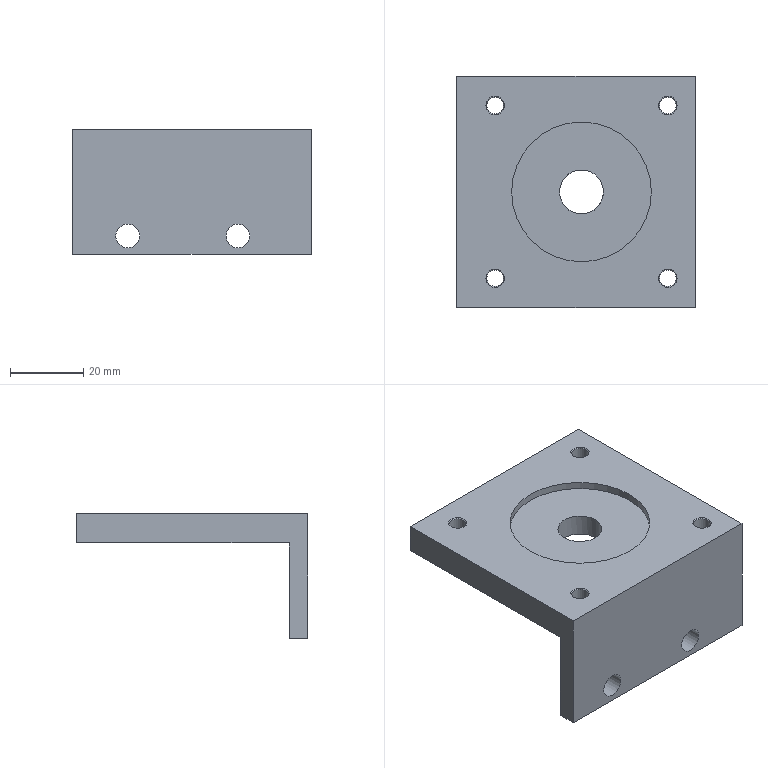Part | NX | features SIMPLE HOLE 7, DATUM_CSYS 5, EXTRUDE 4, SKETCH 4, SYMBOLIC_THREAD 4, HOLE PACKAGE 3 | 1 solid | 25 faces | box 65 x 63 x 34 mm | volume 37407 mm3 | plane 9 | cylinder 8 | cone 8 | commonest cylinder face diameters 4.5 x4 6.5 x2 12 x1 38.1 x1
STEP:
#1=CARTESIAN_POINT('',(35.,5.,0.));
#2=VERTEX_POINT('',#1);
#3=CARTESIAN_POINT('',(-30.,5.,0.));
#4=VERTEX_POINT('',#3);
#5=CARTESIAN_POINT('',(35.,5.,0.));
#6=DIRECTION('',(-1.,0.,0.));
#7=VECTOR('',#6,1000.);
#8=LINE('',#5,#7);
#9=EDGE_CURVE('',#2,#4,#8,.T.);
#10=ORIENTED_EDGE('',*,*,#9,.F.);
#11=CARTESIAN_POINT('',(35.,0.,0.));
#12=VERTEX_POINT('',#11);
#13=CARTESIAN_POINT('',(35.,0.,0.));
#14=DIRECTION('',(0.,1.,0.));
#15=VECTOR('',#14,1000.);
#16=LINE('',#13,#15);
#17=EDGE_CURVE('',#12,#2,#16,.T.);
#18=ORIENTED_EDGE('',*,*,#17,.F.);
#19=CARTESIAN_POINT('',(-30.,0.,0.));
#20=VERTEX_POINT('',#19);
#21=CARTESIAN_POINT('',(30.,0.,0.));
#22=DIRECTION('',(-1.,0.,0.));
#23=VECTOR('',#22,1000.);
#24=LINE('',#21,#23);
#25=EDGE_CURVE('',#12,#20,#24,.T.);
#26=ORIENTED_EDGE('',*,*,#25,.T.);
#27=CARTESIAN_POINT('',(-30.,0.,0.));
#28=DIRECTION('',(0.,1.,0.));
#29=VECTOR('',#28,1000.);
#30=LINE('',#27,#29);
#31=EDGE_CURVE('',#20,#4,#30,.T.);
#32=ORIENTED_EDGE('',*,*,#31,.T.);
#33=EDGE_LOOP('',(#10,#18,#26,#32));
#34=FACE_BOUND('',#33,.T.);
#35=CARTESIAN_POINT('',(30.,0.,0.));
#36=DIRECTION('',(0.,0.,1.));
#37=DIRECTION('',(0.,-1.,0.));
#38=AXIS2_PLACEMENT_3D('',#35,#36,#37);
#39=PLANE('',#38);
#40=ADVANCED_FACE('',(#34),#39,.F.);
#41=CARTESIAN_POINT('',(-30.,5.,26.));
#42=VERTEX_POINT('',#41);
#43=CARTESIAN_POINT('',(-30.,5.,0.));
#44=DIRECTION('',(0.,0.,1.));
#45=VECTOR('',#44,1000.);
#46=LINE('',#43,#45);
#47=EDGE_CURVE('',#4,#42,#46,.T.);
#48=ORIENTED_EDGE('',*,*,#47,.F.);
#49=ORIENTED_EDGE('',*,*,#31,.F.);
#50=CARTESIAN_POINT('',(-30.,0.,34.));
#51=VERTEX_POINT('',#50);
#52=CARTESIAN_POINT('',(-30.,0.,34.));
#53=DIRECTION('',(0.,0.,-1.));
#54=VECTOR('',#53,1000.);
#55=LINE('',#52,#54);
#56=EDGE_CURVE('',#51,#20,#55,.T.);
#57=ORIENTED_EDGE('',*,*,#56,.F.);
#58=CARTESIAN_POINT('',(-30.,63.,34.));
#59=VERTEX_POINT('',#58);
#60=CARTESIAN_POINT('',(-30.,63.,34.));
#61=DIRECTION('',(0.,-1.,0.));
#62=VECTOR('',#61,1000.);
#63=LINE('',#60,#62);
#64=EDGE_CURVE('',#59,#51,#63,.T.);
#65=ORIENTED_EDGE('',*,*,#64,.F.);
#66=CARTESIAN_POINT('',(-30.,63.,26.));
#67=VERTEX_POINT('',#66);
#68=CARTESIAN_POINT('',(-30.,63.,26.));
#69=DIRECTION('',(0.,0.,1.));
#70=VECTOR('',#69,1000.);
#71=LINE('',#68,#70);
#72=EDGE_CURVE('',#67,#59,#71,.T.);
#73=ORIENTED_EDGE('',*,*,#72,.F.);
#74=CARTESIAN_POINT('',(-30.,8.,26.));
#75=DIRECTION('',(0.,1.,0.));
#76=VECTOR('',#75,1000.);
#77=LINE('',#74,#76);
#78=EDGE_CURVE('',#42,#67,#77,.T.);
#79=ORIENTED_EDGE('',*,*,#78,.F.);
#80=EDGE_LOOP('',(#48,#49,#57,#65,#73,#79));
#81=FACE_BOUND('',#80,.T.);
#82=CARTESIAN_POINT('',(-30.,0.,0.));
#83=DIRECTION('',(1.,0.,0.));
#84=DIRECTION('',(0.,0.,-1.));
#85=AXIS2_PLACEMENT_3D('',#82,#83,#84);
#86=PLANE('',#85);
#87=ADVANCED_FACE('',(#81),#86,.F.);
#88=CARTESIAN_POINT('',(35.,5.,26.));
#89=VERTEX_POINT('',#88);
#90=CARTESIAN_POINT('',(35.,5.,26.));
#91=DIRECTION('',(0.,0.,-1.));
#92=VECTOR('',#91,1000.);
#93=LINE('',#90,#92);
#94=EDGE_CURVE('',#89,#2,#93,.T.);
#95=ORIENTED_EDGE('',*,*,#94,.F.);
#96=CARTESIAN_POINT('',(35.,63.,26.));
#97=VERTEX_POINT('',#96);
#98=CARTESIAN_POINT('',(35.,8.,26.));
#99=DIRECTION('',(0.,1.,0.));
#100=VECTOR('',#99,1000.);
#101=LINE('',#98,#100);
#102=EDGE_CURVE('',#89,#97,#101,.T.);
#103=ORIENTED_EDGE('',*,*,#102,.T.);
#104=CARTESIAN_POINT('',(35.,63.,34.));
#105=VERTEX_POINT('',#104);
#106=CARTESIAN_POINT('',(35.,63.,26.));
#107=DIRECTION('',(0.,0.,1.));
#108=VECTOR('',#107,1000.);
#109=LINE('',#106,#108);
#110=EDGE_CURVE('',#97,#105,#109,.T.);
#111=ORIENTED_EDGE('',*,*,#110,.T.);
#112=CARTESIAN_POINT('',(35.,0.,34.));
#113=VERTEX_POINT('',#112);
#114=CARTESIAN_POINT('',(35.,63.,34.));
#115=DIRECTION('',(0.,-1.,0.));
#116=VECTOR('',#115,1000.);
#117=LINE('',#114,#116);
#118=EDGE_CURVE('',#105,#113,#117,.T.);
#119=ORIENTED_EDGE('',*,*,#118,.T.);
#120=CARTESIAN_POINT('',(35.,0.,34.));
#121=DIRECTION('',(0.,0.,-1.));
#122=VECTOR('',#121,1000.);
#123=LINE('',#120,#122);
#124=EDGE_CURVE('',#113,#12,#123,.T.);
#125=ORIENTED_EDGE('',*,*,#124,.T.);
#126=ORIENTED_EDGE('',*,*,#17,.T.);
#127=EDGE_LOOP('',(#95,#103,#111,#119,#125,#126));
#128=FACE_BOUND('',#127,.T.);
#129=CARTESIAN_POINT('',(35.,0.,0.));
#130=DIRECTION('',(1.,0.,0.));
#131=DIRECTION('',(0.,0.,-1.));
#132=AXIS2_PLACEMENT_3D('',#129,#130,#131);
#133=PLANE('',#132);
#134=ADVANCED_FACE('',(#128),#133,.T.);
#135=CARTESIAN_POINT('',(15.,0.,8.25));
#136=VERTEX_POINT('',#135);
#137=CARTESIAN_POINT('',(15.,0.,5.));
#138=DIRECTION('',(0.,1.,0.));
#139=DIRECTION('',(0.,0.,1.));
#140=AXIS2_PLACEMENT_3D('',#137,#138,#139);
#141=CIRCLE('',#140,3.25);
#142=EDGE_CURVE('',#136,#136,#141,.T.);
#143=ORIENTED_EDGE('',*,*,#142,.T.);
#144=EDGE_LOOP('',(#143));
#145=FACE_BOUND('',#144,.T.);
#146=CARTESIAN_POINT('',(-15.,0.,8.25));
#147=VERTEX_POINT('',#146);
#148=CARTESIAN_POINT('',(-15.,0.,5.));
#149=DIRECTION('',(0.,1.,0.));
#150=DIRECTION('',(0.,0.,1.));
#151=AXIS2_PLACEMENT_3D('',#148,#149,#150);
#152=CIRCLE('',#151,3.25);
#153=EDGE_CURVE('',#147,#147,#152,.T.);
#154=ORIENTED_EDGE('',*,*,#153,.T.);
#155=EDGE_LOOP('',(#154));
#156=FACE_BOUND('',#155,.T.);
#157=ORIENTED_EDGE('',*,*,#56,.T.);
#158=ORIENTED_EDGE('',*,*,#25,.F.);
#159=ORIENTED_EDGE('',*,*,#124,.F.);
#160=CARTESIAN_POINT('',(30.,0.,34.));
#161=DIRECTION('',(-1.,0.,0.));
#162=VECTOR('',#161,1000.);
#163=LINE('',#160,#162);
#164=EDGE_CURVE('',#113,#51,#163,.T.);
#165=ORIENTED_EDGE('',*,*,#164,.T.);
#166=EDGE_LOOP('',(#157,#158,#159,#165));
#167=FACE_BOUND('',#166,.T.);
#168=CARTESIAN_POINT('',(30.,0.,34.));
#169=DIRECTION('',(0.,1.,0.));
#170=DIRECTION('',(0.,0.,1.));
#171=AXIS2_PLACEMENT_3D('',#168,#169,#170);
#172=PLANE('',#171);
#173=ADVANCED_FACE('',(#145,#156,#167),#172,.F.);
#174=CARTESIAN_POINT('',(27.55,5.45,26.));
#175=VERTEX_POINT('',#174);
#176=CARTESIAN_POINT('',(27.55,7.95,26.));
#177=DIRECTION('',(0.,0.,1.));
#178=DIRECTION('',(0.,-1.,0.));
#179=AXIS2_PLACEMENT_3D('',#176,#177,#178);
#180=CIRCLE('',#179,2.5);
#181=EDGE_CURVE('',#175,#175,#180,.T.);
#182=ORIENTED_EDGE('',*,*,#181,.T.);
#183=EDGE_LOOP('',(#182));
#184=FACE_BOUND('',#183,.T.);
#185=CARTESIAN_POINT('',(27.55,52.55,26.));
#186=VERTEX_POINT('',#185);
#187=CARTESIAN_POINT('',(27.55,55.05,26.));
#188=DIRECTION('',(0.,0.,1.));
#189=DIRECTION('',(0.,-1.,0.));
#190=AXIS2_PLACEMENT_3D('',#187,#188,#189);
#191=CIRCLE('',#190,2.5);
#192=EDGE_CURVE('',#186,#186,#191,.T.);
#193=ORIENTED_EDGE('',*,*,#192,.T.);
#194=EDGE_LOOP('',(#193));
#195=FACE_BOUND('',#194,.T.);
#196=CARTESIAN_POINT('',(-19.55,52.55,26.));
#197=VERTEX_POINT('',#196);
#198=CARTESIAN_POINT('',(-19.55,55.05,26.));
#199=DIRECTION('',(0.,0.,1.));
#200=DIRECTION('',(0.,-1.,0.));
#201=AXIS2_PLACEMENT_3D('',#198,#199,#200);
#202=CIRCLE('',#201,2.5);
#203=EDGE_CURVE('',#197,#197,#202,.T.);
#204=ORIENTED_EDGE('',*,*,#203,.T.);
#205=EDGE_LOOP('',(#204));
#206=FACE_BOUND('',#205,.T.);
#207=CARTESIAN_POINT('',(-19.55,5.45,26.));
#208=VERTEX_POINT('',#207);
#209=CARTESIAN_POINT('',(-19.55,7.95,26.));
#210=DIRECTION('',(0.,0.,1.));
#211=DIRECTION('',(0.,-1.,0.));
#212=AXIS2_PLACEMENT_3D('',#209,#210,#211);
#213=CIRCLE('',#212,2.5);
#214=EDGE_CURVE('',#208,#208,#213,.T.);
#215=ORIENTED_EDGE('',*,*,#214,.T.);
#216=EDGE_LOOP('',(#215));
#217=FACE_BOUND('',#216,.T.);
#218=CARTESIAN_POINT('',(4.,25.5,26.));
#219=VERTEX_POINT('',#218);
#220=CARTESIAN_POINT('',(4.,31.5,26.));
#221=DIRECTION('',(0.,0.,1.));
#222=DIRECTION('',(0.,-1.,0.));
#223=AXIS2_PLACEMENT_3D('',#220,#221,#222);
#224=CIRCLE('',#223,6.);
#225=EDGE_CURVE('',#219,#219,#224,.T.);
#226=ORIENTED_EDGE('',*,*,#225,.T.);
#227=EDGE_LOOP('',(#226));
#228=FACE_BOUND('',#227,.T.);
#229=ORIENTED_EDGE('',*,*,#78,.T.);
#230=CARTESIAN_POINT('',(30.,63.,26.));
#231=DIRECTION('',(-1.,0.,0.));
#232=VECTOR('',#231,1000.);
#233=LINE('',#230,#232);
#234=EDGE_CURVE('',#97,#67,#233,.T.);
#235=ORIENTED_EDGE('',*,*,#234,.F.);
#236=ORIENTED_EDGE('',*,*,#102,.F.);
#237=CARTESIAN_POINT('',(-30.,5.,26.));
#238=DIRECTION('',(1.,0.,0.));
#239=VECTOR('',#238,1000.);
#240=LINE('',#237,#239);
#241=EDGE_CURVE('',#42,#89,#240,.T.);
#242=ORIENTED_EDGE('',*,*,#241,.F.);
#243=EDGE_LOOP('',(#229,#235,#236,#242));
#244=FACE_BOUND('',#243,.T.);
#245=CARTESIAN_POINT('',(30.,8.,26.));
#246=DIRECTION('',(0.,0.,1.));
#247=DIRECTION('',(0.,-1.,0.));
#248=AXIS2_PLACEMENT_3D('',#245,#246,#247);
#249=PLANE('',#248);
#250=ADVANCED_FACE('',(#184,#195,#206,#217,#228,#244),#249,.F.);
#251=ORIENTED_EDGE('',*,*,#72,.T.);
#252=CARTESIAN_POINT('',(30.,63.,34.));
#253=DIRECTION('',(-1.,0.,0.));
#254=VECTOR('',#253,1000.);
#255=LINE('',#252,#254);
#256=EDGE_CURVE('',#105,#59,#255,.T.);
#257=ORIENTED_EDGE('',*,*,#256,.F.);
#258=ORIENTED_EDGE('',*,*,#110,.F.);
#259=ORIENTED_EDGE('',*,*,#234,.T.);
#260=EDGE_LOOP('',(#251,#257,#258,#259));
#261=FACE_BOUND('',#260,.T.);
#262=CARTESIAN_POINT('',(30.,63.,26.));
#263=DIRECTION('',(0.,-1.,0.));
#264=DIRECTION('',(0.,0.,-1.));
#265=AXIS2_PLACEMENT_3D('',#262,#263,#264);
#266=PLANE('',#265);
#267=ADVANCED_FACE('',(#261),#266,.F.);
#268=CARTESIAN_POINT('',(25.05,7.95,34.));
#269=VERTEX_POINT('',#268);
#270=CARTESIAN_POINT('',(27.55,7.95,34.));
#271=DIRECTION('',(0.,0.,-1.));
#272=DIRECTION('',(-1.,0.,0.));
#273=AXIS2_PLACEMENT_3D('',#270,#271,#272);
#274=CIRCLE('',#273,2.5);
#275=EDGE_CURVE('',#269,#269,#274,.T.);
#276=ORIENTED_EDGE('',*,*,#275,.T.);
#277=EDGE_LOOP('',(#276));
#278=FACE_BOUND('',#277,.T.);
#279=CARTESIAN_POINT('',(25.05,55.05,34.));
#280=VERTEX_POINT('',#279);
#281=CARTESIAN_POINT('',(27.55,55.05,34.));
#282=DIRECTION('',(0.,0.,-1.));
#283=DIRECTION('',(-1.,0.,0.));
#284=AXIS2_PLACEMENT_3D('',#281,#282,#283);
#285=CIRCLE('',#284,2.5);
#286=EDGE_CURVE('',#280,#280,#285,.T.);
#287=ORIENTED_EDGE('',*,*,#286,.T.);
#288=EDGE_LOOP('',(#287));
#289=FACE_BOUND('',#288,.T.);
#290=CARTESIAN_POINT('',(-22.05,55.05,34.));
#291=VERTEX_POINT('',#290);
#292=CARTESIAN_POINT('',(-19.55,55.05,34.));
#293=DIRECTION('',(0.,0.,-1.));
#294=DIRECTION('',(-1.,0.,0.));
#295=AXIS2_PLACEMENT_3D('',#292,#293,#294);
#296=CIRCLE('',#295,2.5);
#297=EDGE_CURVE('',#291,#291,#296,.T.);
#298=ORIENTED_EDGE('',*,*,#297,.T.);
#299=EDGE_LOOP('',(#298));
#300=FACE_BOUND('',#299,.T.);
#301=CARTESIAN_POINT('',(-22.05,7.95,34.));
#302=VERTEX_POINT('',#301);
#303=CARTESIAN_POINT('',(-19.55,7.95,34.));
#304=DIRECTION('',(0.,0.,-1.));
#305=DIRECTION('',(-1.,0.,0.));
#306=AXIS2_PLACEMENT_3D('',#303,#304,#305);
#307=CIRCLE('',#306,2.5);
#308=EDGE_CURVE('',#302,#302,#307,.T.);
#309=ORIENTED_EDGE('',*,*,#308,.T.);
#310=EDGE_LOOP('',(#309));
#311=FACE_BOUND('',#310,.T.);
#312=CARTESIAN_POINT('',(4.,50.55,34.));
#313=VERTEX_POINT('',#312);
#314=CARTESIAN_POINT('',(4.,31.5,34.));
#315=DIRECTION('',(0.,0.,1.));
#316=DIRECTION('',(0.,1.,0.));
#317=AXIS2_PLACEMENT_3D('',#314,#315,#316);
#318=CIRCLE('',#317,19.05);
#319=EDGE_CURVE('',#313,#313,#318,.T.);
#320=ORIENTED_EDGE('',*,*,#319,.F.);
#321=EDGE_LOOP('',(#320));
#322=FACE_BOUND('',#321,.T.);
#323=ORIENTED_EDGE('',*,*,#64,.T.);
#324=ORIENTED_EDGE('',*,*,#164,.F.);
#325=ORIENTED_EDGE('',*,*,#118,.F.);
#326=ORIENTED_EDGE('',*,*,#256,.T.);
#327=EDGE_LOOP('',(#323,#324,#325,#326));
#328=FACE_BOUND('',#327,.T.);
#329=CARTESIAN_POINT('',(30.,63.,34.));
#330=DIRECTION('',(0.,0.,-1.));
#331=DIRECTION('',(-1.,0.,0.));
#332=AXIS2_PLACEMENT_3D('',#329,#330,#331);
#333=PLANE('',#332);
#334=ADVANCED_FACE('',(#278,#289,#300,#311,#322,#328),#333,.F.);
#335=CARTESIAN_POINT('',(4.,50.55,32.));
#336=VERTEX_POINT('',#335);
#337=CARTESIAN_POINT('',(4.,31.5,32.));
#338=DIRECTION('',(0.,0.,1.));
#339=DIRECTION('',(0.,1.,0.));
#340=AXIS2_PLACEMENT_3D('',#337,#338,#339);
#341=CIRCLE('',#340,19.05);
#342=EDGE_CURVE('',#336,#336,#341,.F.);
#343=ORIENTED_EDGE('',*,*,#342,.T.);
#344=EDGE_LOOP('',(#343));
#345=FACE_BOUND('',#344,.T.);
#346=ORIENTED_EDGE('',*,*,#319,.T.);
#347=EDGE_LOOP('',(#346));
#348=FACE_BOUND('',#347,.T.);
#349=CARTESIAN_POINT('',(4.,31.5,32.));
#350=DIRECTION('',(0.,0.,1.));
#351=DIRECTION('',(1.,0.,0.));
#352=AXIS2_PLACEMENT_3D('',#349,#350,#351);
#353=CYLINDRICAL_SURFACE('',#352,19.05);
#354=ADVANCED_FACE('',(#345,#348),#353,.F.);
#355=CARTESIAN_POINT('',(-2.,31.5,32.));
#356=VERTEX_POINT('',#355);
#357=CARTESIAN_POINT('',(4.,31.5,32.));
#358=DIRECTION('',(0.,0.,-1.));
#359=DIRECTION('',(-1.,0.,0.));
#360=AXIS2_PLACEMENT_3D('',#357,#358,#359);
#361=CIRCLE('',#360,6.);
#362=EDGE_CURVE('',#356,#356,#361,.T.);
#363=ORIENTED_EDGE('',*,*,#362,.T.);
#364=EDGE_LOOP('',(#363));
#365=FACE_BOUND('',#364,.T.);
#366=ORIENTED_EDGE('',*,*,#342,.F.);
#367=EDGE_LOOP('',(#366));
#368=FACE_BOUND('',#367,.T.);
#369=CARTESIAN_POINT('',(4.,31.5,32.));
#370=DIRECTION('',(0.,0.,1.));
#371=DIRECTION('',(1.,0.,0.));
#372=AXIS2_PLACEMENT_3D('',#369,#370,#371);
#373=PLANE('',#372);
#374=ADVANCED_FACE('',(#365,#368),#373,.T.);
#375=ORIENTED_EDGE('',*,*,#362,.F.);
#376=EDGE_LOOP('',(#375));
#377=FACE_BOUND('',#376,.T.);
#378=ORIENTED_EDGE('',*,*,#225,.F.);
#379=EDGE_LOOP('',(#378));
#380=FACE_BOUND('',#379,.T.);
#381=CARTESIAN_POINT('',(4.,31.5,32.));
#382=DIRECTION('',(0.,0.,-1.));
#383=DIRECTION('',(-1.,0.,0.));
#384=AXIS2_PLACEMENT_3D('',#381,#382,#383);
#385=CYLINDRICAL_SURFACE('',#384,6.);
#386=ADVANCED_FACE('',(#377,#380),#385,.F.);
#387=CARTESIAN_POINT('',(15.,5.,8.25));
#388=VERTEX_POINT('',#387);
#389=CARTESIAN_POINT('',(15.,5.,5.));
#390=DIRECTION('',(0.,1.,0.));
#391=DIRECTION('',(0.,0.,1.));
#392=AXIS2_PLACEMENT_3D('',#389,#390,#391);
#393=CIRCLE('',#392,3.25);
#394=EDGE_CURVE('',#388,#388,#393,.T.);
#395=ORIENTED_EDGE('',*,*,#394,.F.);
#396=EDGE_LOOP('',(#395));
#397=FACE_BOUND('',#396,.T.);
#398=CARTESIAN_POINT('',(-15.,5.,8.25));
#399=VERTEX_POINT('',#398);
#400=CARTESIAN_POINT('',(-15.,5.,5.));
#401=DIRECTION('',(0.,1.,0.));
#402=DIRECTION('',(0.,0.,1.));
#403=AXIS2_PLACEMENT_3D('',#400,#401,#402);
#404=CIRCLE('',#403,3.25);
#405=EDGE_CURVE('',#399,#399,#404,.T.);
#406=ORIENTED_EDGE('',*,*,#405,.F.);
#407=EDGE_LOOP('',(#406));
#408=FACE_BOUND('',#407,.T.);
#409=ORIENTED_EDGE('',*,*,#47,.T.);
#410=ORIENTED_EDGE('',*,*,#241,.T.);
#411=ORIENTED_EDGE('',*,*,#94,.T.);
#412=ORIENTED_EDGE('',*,*,#9,.T.);
#413=EDGE_LOOP('',(#409,#410,#411,#412));
#414=FACE_BOUND('',#413,.T.);
#415=CARTESIAN_POINT('',(0.,5.,0.));
#416=DIRECTION('',(0.,1.,0.));
#417=DIRECTION('',(0.,0.,1.));
#418=AXIS2_PLACEMENT_3D('',#415,#416,#417);
#419=PLANE('',#418);
#420=ADVANCED_FACE('',(#397,#408,#414),#419,.T.);
#421=CARTESIAN_POINT('',(-17.3,7.95,26.25));
#422=VERTEX_POINT('',#421);
#423=CARTESIAN_POINT('',(-19.55,7.95,26.25));
#424=DIRECTION('',(0.,0.,1.));
#425=DIRECTION('',(1.,0.,0.));
#426=AXIS2_PLACEMENT_3D('',#423,#424,#425);
#427=CIRCLE('',#426,2.25);
#428=EDGE_CURVE('',#422,#422,#427,.F.);
#429=ORIENTED_EDGE('',*,*,#428,.T.);
#430=EDGE_LOOP('',(#429));
#431=FACE_BOUND('',#430,.T.);
#432=CARTESIAN_POINT('',(-21.8,7.95,33.75));
#433=VERTEX_POINT('',#432);
#434=CARTESIAN_POINT('',(-19.55,7.95,33.75));
#435=DIRECTION('',(0.,0.,-1.));
#436=DIRECTION('',(-1.,0.,0.));
#437=AXIS2_PLACEMENT_3D('',#434,#435,#436);
#438=CIRCLE('',#437,2.25);
#439=EDGE_CURVE('',#433,#433,#438,.F.);
#440=ORIENTED_EDGE('',*,*,#439,.T.);
#441=EDGE_LOOP('',(#440));
#442=FACE_BOUND('',#441,.T.);
#443=CARTESIAN_POINT('',(-19.55,7.95,34.));
#444=DIRECTION('',(0.,0.,-1.));
#445=DIRECTION('',(-1.,0.,0.));
#446=AXIS2_PLACEMENT_3D('',#443,#444,#445);
#447=CYLINDRICAL_SURFACE('',#446,2.25);
#448=ADVANCED_FACE('',(#431,#442),#447,.F.);
#449=ORIENTED_EDGE('',*,*,#439,.F.);
#450=EDGE_LOOP('',(#449));
#451=FACE_BOUND('',#450,.T.);
#452=ORIENTED_EDGE('',*,*,#308,.F.);
#453=EDGE_LOOP('',(#452));
#454=FACE_BOUND('',#453,.T.);
#455=CARTESIAN_POINT('',(-19.55,7.95,34.));
#456=DIRECTION('',(0.,0.,1.));
#457=DIRECTION('',(1.,0.,0.));
#458=AXIS2_PLACEMENT_3D('',#455,#456,#457);
#459=CONICAL_SURFACE('',#458,2.5,0.7854);
#460=ADVANCED_FACE('',(#451,#454),#459,.F.);
#461=ORIENTED_EDGE('',*,*,#428,.F.);
#462=EDGE_LOOP('',(#461));
#463=FACE_BOUND('',#462,.T.);
#464=ORIENTED_EDGE('',*,*,#214,.F.);
#465=EDGE_LOOP('',(#464));
#466=FACE_BOUND('',#465,.T.);
#467=CARTESIAN_POINT('',(-19.55,7.95,26.));
#468=DIRECTION('',(0.,0.,-1.));
#469=DIRECTION('',(-1.,0.,0.));
#470=AXIS2_PLACEMENT_3D('',#467,#468,#469);
#471=CONICAL_SURFACE('',#470,2.5,0.7854);
#472=ADVANCED_FACE('',(#463,#466),#471,.F.);
#473=CARTESIAN_POINT('',(-17.3,55.05,26.25));
#474=VERTEX_POINT('',#473);
#475=CARTESIAN_POINT('',(-19.55,55.05,26.25));
#476=DIRECTION('',(0.,0.,1.));
#477=DIRECTION('',(1.,0.,0.));
#478=AXIS2_PLACEMENT_3D('',#475,#476,#477);
#479=CIRCLE('',#478,2.25);
#480=EDGE_CURVE('',#474,#474,#479,.F.);
#481=ORIENTED_EDGE('',*,*,#480,.T.);
#482=EDGE_LOOP('',(#481));
#483=FACE_BOUND('',#482,.T.);
#484=CARTESIAN_POINT('',(-21.8,55.05,33.75));
#485=VERTEX_POINT('',#484);
#486=CARTESIAN_POINT('',(-19.55,55.05,33.75));
#487=DIRECTION('',(0.,0.,-1.));
#488=DIRECTION('',(-1.,0.,0.));
#489=AXIS2_PLACEMENT_3D('',#486,#487,#488);
#490=CIRCLE('',#489,2.25);
#491=EDGE_CURVE('',#485,#485,#490,.F.);
#492=ORIENTED_EDGE('',*,*,#491,.T.);
#493=EDGE_LOOP('',(#492));
#494=FACE_BOUND('',#493,.T.);
#495=CARTESIAN_POINT('',(-19.55,55.05,34.));
#496=DIRECTION('',(0.,0.,-1.));
#497=DIRECTION('',(-1.,0.,0.));
#498=AXIS2_PLACEMENT_3D('',#495,#496,#497);
#499=CYLINDRICAL_SURFACE('',#498,2.25);
#500=ADVANCED_FACE('',(#483,#494),#499,.F.);
#501=ORIENTED_EDGE('',*,*,#491,.F.);
#502=EDGE_LOOP('',(#501));
#503=FACE_BOUND('',#502,.T.);
#504=ORIENTED_EDGE('',*,*,#297,.F.);
#505=EDGE_LOOP('',(#504));
#506=FACE_BOUND('',#505,.T.);
#507=CARTESIAN_POINT('',(-19.55,55.05,34.));
#508=DIRECTION('',(0.,0.,1.));
#509=DIRECTION('',(1.,0.,0.));
#510=AXIS2_PLACEMENT_3D('',#507,#508,#509);
#511=CONICAL_SURFACE('',#510,2.5,0.7854);
#512=ADVANCED_FACE('',(#503,#506),#511,.F.);
#513=ORIENTED_EDGE('',*,*,#480,.F.);
#514=EDGE_LOOP('',(#513));
#515=FACE_BOUND('',#514,.T.);
#516=ORIENTED_EDGE('',*,*,#203,.F.);
#517=EDGE_LOOP('',(#516));
#518=FACE_BOUND('',#517,.T.);
#519=CARTESIAN_POINT('',(-19.55,55.05,26.));
#520=DIRECTION('',(0.,0.,-1.));
#521=DIRECTION('',(-1.,0.,0.));
#522=AXIS2_PLACEMENT_3D('',#519,#520,#521);
#523=CONICAL_SURFACE('',#522,2.5,0.7854);
#524=ADVANCED_FACE('',(#515,#518),#523,.F.);
#525=CARTESIAN_POINT('',(29.8,55.05,26.25));
#526=VERTEX_POINT('',#525);
#527=CARTESIAN_POINT('',(27.55,55.05,26.25));
#528=DIRECTION('',(0.,0.,1.));
#529=DIRECTION('',(1.,0.,0.));
#530=AXIS2_PLACEMENT_3D('',#527,#528,#529);
#531=CIRCLE('',#530,2.25);
#532=EDGE_CURVE('',#526,#526,#531,.F.);
#533=ORIENTED_EDGE('',*,*,#532,.T.);
#534=EDGE_LOOP('',(#533));
#535=FACE_BOUND('',#534,.T.);
#536=CARTESIAN_POINT('',(25.3,55.05,33.75));
#537=VERTEX_POINT('',#536);
#538=CARTESIAN_POINT('',(27.55,55.05,33.75));
#539=DIRECTION('',(0.,0.,-1.));
#540=DIRECTION('',(-1.,0.,0.));
#541=AXIS2_PLACEMENT_3D('',#538,#539,#540);
#542=CIRCLE('',#541,2.25);
#543=EDGE_CURVE('',#537,#537,#542,.F.);
#544=ORIENTED_EDGE('',*,*,#543,.T.);
#545=EDGE_LOOP('',(#544));
#546=FACE_BOUND('',#545,.T.);
#547=CARTESIAN_POINT('',(27.55,55.05,34.));
#548=DIRECTION('',(0.,0.,-1.));
#549=DIRECTION('',(-1.,0.,0.));
#550=AXIS2_PLACEMENT_3D('',#547,#548,#549);
#551=CYLINDRICAL_SURFACE('',#550,2.25);
#552=ADVANCED_FACE('',(#535,#546),#551,.F.);
#553=ORIENTED_EDGE('',*,*,#543,.F.);
#554=EDGE_LOOP('',(#553));
#555=FACE_BOUND('',#554,.T.);
#556=ORIENTED_EDGE('',*,*,#286,.F.);
#557=EDGE_LOOP('',(#556));
#558=FACE_BOUND('',#557,.T.);
#559=CARTESIAN_POINT('',(27.55,55.05,34.));
#560=DIRECTION('',(0.,0.,1.));
#561=DIRECTION('',(1.,0.,0.));
#562=AXIS2_PLACEMENT_3D('',#559,#560,#561);
#563=CONICAL_SURFACE('',#562,2.5,0.7854);
#564=ADVANCED_FACE('',(#555,#558),#563,.F.);
#565=ORIENTED_EDGE('',*,*,#532,.F.);
#566=EDGE_LOOP('',(#565));
#567=FACE_BOUND('',#566,.T.);
#568=ORIENTED_EDGE('',*,*,#192,.F.);
#569=EDGE_LOOP('',(#568));
#570=FACE_BOUND('',#569,.T.);
#571=CARTESIAN_POINT('',(27.55,55.05,26.));
#572=DIRECTION('',(0.,0.,-1.));
#573=DIRECTION('',(-1.,0.,0.));
#574=AXIS2_PLACEMENT_3D('',#571,#572,#573);
#575=CONICAL_SURFACE('',#574,2.5,0.7854);
#576=ADVANCED_FACE('',(#567,#570),#575,.F.);
#577=CARTESIAN_POINT('',(29.8,7.95,26.25));
#578=VERTEX_POINT('',#577);
#579=CARTESIAN_POINT('',(27.55,7.95,26.25));
#580=DIRECTION('',(0.,0.,1.));
#581=DIRECTION('',(1.,0.,0.));
#582=AXIS2_PLACEMENT_3D('',#579,#580,#581);
#583=CIRCLE('',#582,2.25);
#584=EDGE_CURVE('',#578,#578,#583,.F.);
#585=ORIENTED_EDGE('',*,*,#584,.T.);
#586=EDGE_LOOP('',(#585));
#587=FACE_BOUND('',#586,.T.);
#588=CARTESIAN_POINT('',(25.3,7.95,33.75));
#589=VERTEX_POINT('',#588);
#590=CARTESIAN_POINT('',(27.55,7.95,33.75));
#591=DIRECTION('',(0.,0.,-1.));
#592=DIRECTION('',(-1.,0.,0.));
#593=AXIS2_PLACEMENT_3D('',#590,#591,#592);
#594=CIRCLE('',#593,2.25);
#595=EDGE_CURVE('',#589,#589,#594,.F.);
#596=ORIENTED_EDGE('',*,*,#595,.T.);
#597=EDGE_LOOP('',(#596));
#598=FACE_BOUND('',#597,.T.);
#599=CARTESIAN_POINT('',(27.55,7.95,34.));
#600=DIRECTION('',(0.,0.,-1.));
#601=DIRECTION('',(-1.,0.,0.));
#602=AXIS2_PLACEMENT_3D('',#599,#600,#601);
#603=CYLINDRICAL_SURFACE('',#602,2.25);
#604=ADVANCED_FACE('',(#587,#598),#603,.F.);
#605=ORIENTED_EDGE('',*,*,#595,.F.);
#606=EDGE_LOOP('',(#605));
#607=FACE_BOUND('',#606,.T.);
#608=ORIENTED_EDGE('',*,*,#275,.F.);
#609=EDGE_LOOP('',(#608));
#610=FACE_BOUND('',#609,.T.);
#611=CARTESIAN_POINT('',(27.55,7.95,34.));
#612=DIRECTION('',(0.,0.,1.));
#613=DIRECTION('',(1.,0.,0.));
#614=AXIS2_PLACEMENT_3D('',#611,#612,#613);
#615=CONICAL_SURFACE('',#614,2.5,0.7854);
#616=ADVANCED_FACE('',(#607,#610),#615,.F.);
#617=ORIENTED_EDGE('',*,*,#584,.F.);
#618=EDGE_LOOP('',(#617));
#619=FACE_BOUND('',#618,.T.);
#620=ORIENTED_EDGE('',*,*,#181,.F.);
#621=EDGE_LOOP('',(#620));
#622=FACE_BOUND('',#621,.T.);
#623=CARTESIAN_POINT('',(27.55,7.95,26.));
#624=DIRECTION('',(0.,0.,-1.));
#625=DIRECTION('',(-1.,0.,0.));
#626=AXIS2_PLACEMENT_3D('',#623,#624,#625);
#627=CONICAL_SURFACE('',#626,2.5,0.7854);
#628=ADVANCED_FACE('',(#619,#622),#627,.F.);
#629=ORIENTED_EDGE('',*,*,#405,.T.);
#630=EDGE_LOOP('',(#629));
#631=FACE_BOUND('',#630,.T.);
#632=ORIENTED_EDGE('',*,*,#153,.F.);
#633=EDGE_LOOP('',(#632));
#634=FACE_BOUND('',#633,.T.);
#635=CARTESIAN_POINT('',(-15.,0.,5.));
#636=DIRECTION('',(0.,1.,0.));
#637=DIRECTION('',(0.,0.,1.));
#638=AXIS2_PLACEMENT_3D('',#635,#636,#637);
#639=CYLINDRICAL_SURFACE('',#638,3.25);
#640=ADVANCED_FACE('',(#631,#634),#639,.F.);
#641=ORIENTED_EDGE('',*,*,#394,.T.);
#642=EDGE_LOOP('',(#641));
#643=FACE_BOUND('',#642,.T.);
#644=ORIENTED_EDGE('',*,*,#142,.F.);
#645=EDGE_LOOP('',(#644));
#646=FACE_BOUND('',#645,.T.);
#647=CARTESIAN_POINT('',(15.,0.,5.));
#648=DIRECTION('',(0.,1.,0.));
#649=DIRECTION('',(0.,0.,1.));
#650=AXIS2_PLACEMENT_3D('',#647,#648,#649);
#651=CYLINDRICAL_SURFACE('',#650,3.25);
#652=ADVANCED_FACE('',(#643,#646),#651,.F.);
#653=CLOSED_SHELL('',(#40,#87,#134,#173,#250,#267,#334,#354,#374,#386,#420,#448,#460,#472,#500,#512,#524,#552,#564,#576,#604,#616,#628,#640,#652));
#654=MANIFOLD_SOLID_BREP('',#653);
#655=(LENGTH_UNIT()NAMED_UNIT(*)SI_UNIT(.MILLI.,.METRE.));
#656=UNCERTAINTY_MEASURE_WITH_UNIT(LENGTH_MEASURE(0.00001),#655,'','');
#657=(NAMED_UNIT(*)PLANE_ANGLE_UNIT()SI_UNIT($,.RADIAN.));
#658=(NAMED_UNIT(*)SI_UNIT($,.STERADIAN.)SOLID_ANGLE_UNIT());
#659=(GEOMETRIC_REPRESENTATION_CONTEXT(3)GLOBAL_UNCERTAINTY_ASSIGNED_CONTEXT((#656))GLOBAL_UNIT_ASSIGNED_CONTEXT((#655,#657,#658))REPRESENTATION_CONTEXT('',''));
#660=ADVANCED_BREP_SHAPE_REPRESENTATION('',(#654),#659);